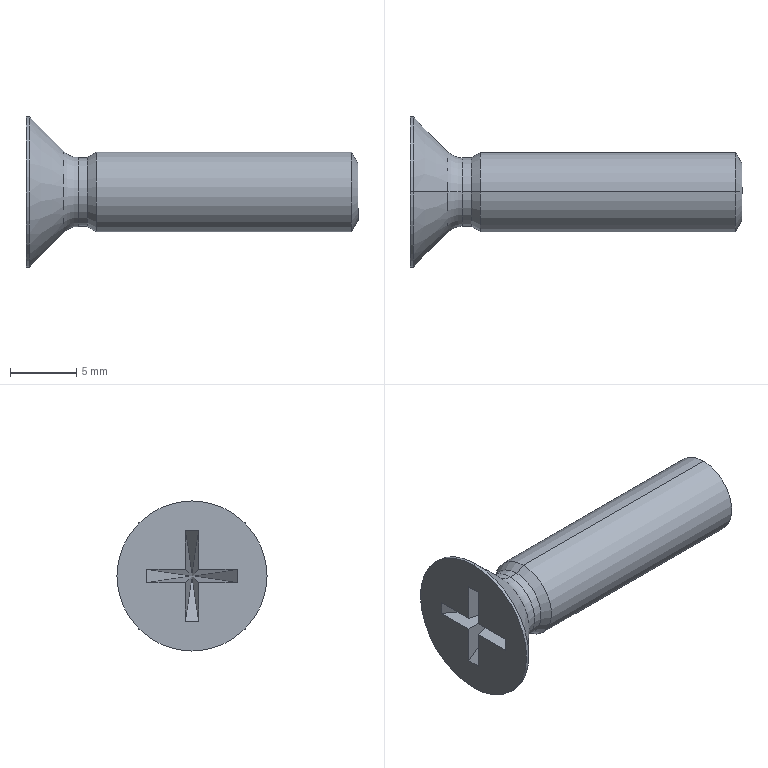Part | SolidWorks | features BaseBody 1 | 1 solid | 28 faces | box 25 x 11.3 x 11.3 mm | volume 779.668 mm3 | plane 14 | cone 6 | cylinder 6 | torus 2 | commonest cylinder face diameters 5.196 x2 6 x2 11.3 x2
STEP:
#1=CARTESIAN_POINT('',(0.,3.4,0.5));
#2=VERTEX_POINT('',#1);
#3=CARTESIAN_POINT('',(3.5,0.,0.));
#4=VERTEX_POINT('',#3);
#5=CARTESIAN_POINT('',(0.,3.4,0.5));
#6=DIRECTION('',(0.7135,-0.6932,-0.1019));
#7=VECTOR('',#6,1000.);
#8=LINE('',#5,#7);
#9=EDGE_CURVE('',#2,#4,#8,.T.);
#10=ORIENTED_EDGE('',*,*,#9,.F.);
#11=CARTESIAN_POINT('',(0.,3.4,-0.5));
#12=VERTEX_POINT('',#11);
#13=CARTESIAN_POINT('',(0.,3.4,0.5));
#14=DIRECTION('',(0.,0.,-1.));
#15=VECTOR('',#14,1000.);
#16=LINE('',#13,#15);
#17=EDGE_CURVE('',#2,#12,#16,.T.);
#18=ORIENTED_EDGE('',*,*,#17,.T.);
#19=CARTESIAN_POINT('',(0.,3.4,-0.5));
#20=DIRECTION('',(0.7135,-0.6932,0.1019));
#21=VECTOR('',#20,1000.);
#22=LINE('',#19,#21);
#23=EDGE_CURVE('',#12,#4,#22,.T.);
#24=ORIENTED_EDGE('',*,*,#23,.T.);
#25=EDGE_LOOP('',(#10,#18,#24));
#26=FACE_OUTER_BOUND('',#25,.T.);
#27=CARTESIAN_POINT('',(0.,3.4,0.5));
#28=DIRECTION('',(0.6968,0.7173,0.));
#29=DIRECTION('',(0.,0.,-1.));
#30=AXIS2_PLACEMENT_3D('',#27,#28,#29);
#31=PLANE('',#30);
#32=ADVANCED_FACE('',(#26),#31,.F.);
#33=ORIENTED_EDGE('',*,*,#23,.F.);
#34=CARTESIAN_POINT('',(0.,0.5,-0.5));
#35=VERTEX_POINT('',#34);
#36=CARTESIAN_POINT('',(0.,3.4,-0.5));
#37=DIRECTION('',(0.,-1.,0.));
#38=VECTOR('',#37,1000.);
#39=LINE('',#36,#38);
#40=EDGE_CURVE('',#12,#35,#39,.T.);
#41=ORIENTED_EDGE('',*,*,#40,.T.);
#42=CARTESIAN_POINT('',(3.5,0.,0.));
#43=DIRECTION('',(-0.9802,0.14,-0.14));
#44=VECTOR('',#43,1000.);
#45=LINE('',#42,#44);
#46=EDGE_CURVE('',#4,#35,#45,.T.);
#47=ORIENTED_EDGE('',*,*,#46,.F.);
#48=EDGE_LOOP('',(#33,#41,#47));
#49=FACE_OUTER_BOUND('',#48,.T.);
#50=CARTESIAN_POINT('',(3.5,0.,0.));
#51=DIRECTION('',(-0.1414,0.,0.9899));
#52=DIRECTION('',(0.,1.,0.));
#53=AXIS2_PLACEMENT_3D('',#50,#51,#52);
#54=PLANE('',#53);
#55=ADVANCED_FACE('',(#49),#54,.T.);
#56=CARTESIAN_POINT('',(0.,0.5,0.5));
#57=VERTEX_POINT('',#56);
#58=CARTESIAN_POINT('',(0.,3.4,0.5));
#59=DIRECTION('',(0.,1.,0.));
#60=VECTOR('',#59,1000.);
#61=LINE('',#58,#60);
#62=EDGE_CURVE('',#57,#2,#61,.T.);
#63=ORIENTED_EDGE('',*,*,#62,.T.);
#64=ORIENTED_EDGE('',*,*,#9,.T.);
#65=CARTESIAN_POINT('',(3.5,0.,0.));
#66=DIRECTION('',(0.9802,-0.14,-0.14));
#67=VECTOR('',#66,1000.);
#68=LINE('',#65,#67);
#69=EDGE_CURVE('',#57,#4,#68,.T.);
#70=ORIENTED_EDGE('',*,*,#69,.F.);
#71=EDGE_LOOP('',(#63,#64,#70));
#72=FACE_OUTER_BOUND('',#71,.T.);
#73=CARTESIAN_POINT('',(3.5,0.,0.));
#74=DIRECTION('',(-0.1414,0.,-0.9899));
#75=DIRECTION('',(-0.9899,0.,0.1414));
#76=AXIS2_PLACEMENT_3D('',#73,#74,#75);
#77=PLANE('',#76);
#78=ADVANCED_FACE('',(#72),#77,.T.);
#79=CARTESIAN_POINT('',(0.,-3.4,-0.5));
#80=VERTEX_POINT('',#79);
#81=CARTESIAN_POINT('',(0.,-3.4,-0.5));
#82=DIRECTION('',(0.7135,0.6932,0.1019));
#83=VECTOR('',#82,1000.);
#84=LINE('',#81,#83);
#85=EDGE_CURVE('',#80,#4,#84,.T.);
#86=ORIENTED_EDGE('',*,*,#85,.F.);
#87=CARTESIAN_POINT('',(0.,-3.4,0.5));
#88=VERTEX_POINT('',#87);
#89=CARTESIAN_POINT('',(0.,-3.4,0.5));
#90=DIRECTION('',(0.,0.,1.));
#91=VECTOR('',#90,1000.);
#92=LINE('',#89,#91);
#93=EDGE_CURVE('',#80,#88,#92,.T.);
#94=ORIENTED_EDGE('',*,*,#93,.T.);
#95=CARTESIAN_POINT('',(0.,-3.4,0.5));
#96=DIRECTION('',(0.7135,0.6932,-0.1019));
#97=VECTOR('',#96,1000.);
#98=LINE('',#95,#97);
#99=EDGE_CURVE('',#88,#4,#98,.T.);
#100=ORIENTED_EDGE('',*,*,#99,.T.);
#101=EDGE_LOOP('',(#86,#94,#100));
#102=FACE_OUTER_BOUND('',#101,.T.);
#103=CARTESIAN_POINT('',(0.,-3.4,-0.5));
#104=DIRECTION('',(0.6968,-0.7173,0.));
#105=DIRECTION('',(0.,0.,-1.));
#106=AXIS2_PLACEMENT_3D('',#103,#104,#105);
#107=PLANE('',#106);
#108=ADVANCED_FACE('',(#102),#107,.F.);
#109=CARTESIAN_POINT('',(0.,-0.5,-0.5));
#110=VERTEX_POINT('',#109);
#111=CARTESIAN_POINT('',(0.,3.4,-0.5));
#112=DIRECTION('',(0.,-1.,0.));
#113=VECTOR('',#112,1000.);
#114=LINE('',#111,#113);
#115=EDGE_CURVE('',#110,#80,#114,.T.);
#116=ORIENTED_EDGE('',*,*,#115,.T.);
#117=ORIENTED_EDGE('',*,*,#85,.T.);
#118=CARTESIAN_POINT('',(3.5,0.,0.));
#119=DIRECTION('',(0.9802,0.14,0.14));
#120=VECTOR('',#119,1000.);
#121=LINE('',#118,#120);
#122=EDGE_CURVE('',#110,#4,#121,.T.);
#123=ORIENTED_EDGE('',*,*,#122,.F.);
#124=EDGE_LOOP('',(#116,#117,#123));
#125=FACE_OUTER_BOUND('',#124,.T.);
#126=CARTESIAN_POINT('',(3.5,0.,0.));
#127=DIRECTION('',(-0.1414,0.,0.9899));
#128=DIRECTION('',(0.,1.,0.));
#129=AXIS2_PLACEMENT_3D('',#126,#127,#128);
#130=PLANE('',#129);
#131=ADVANCED_FACE('',(#125),#130,.T.);
#132=ORIENTED_EDGE('',*,*,#99,.F.);
#133=CARTESIAN_POINT('',(0.,-0.5,0.5));
#134=VERTEX_POINT('',#133);
#135=CARTESIAN_POINT('',(0.,3.4,0.5));
#136=DIRECTION('',(0.,1.,0.));
#137=VECTOR('',#136,1000.);
#138=LINE('',#135,#137);
#139=EDGE_CURVE('',#88,#134,#138,.T.);
#140=ORIENTED_EDGE('',*,*,#139,.T.);
#141=CARTESIAN_POINT('',(3.5,0.,0.));
#142=DIRECTION('',(-0.9802,-0.14,0.14));
#143=VECTOR('',#142,1000.);
#144=LINE('',#141,#143);
#145=EDGE_CURVE('',#4,#134,#144,.T.);
#146=ORIENTED_EDGE('',*,*,#145,.F.);
#147=EDGE_LOOP('',(#132,#140,#146));
#148=FACE_OUTER_BOUND('',#147,.T.);
#149=CARTESIAN_POINT('',(3.5,0.,0.));
#150=DIRECTION('',(-0.1414,0.,-0.9899));
#151=DIRECTION('',(-0.9899,0.,0.1414));
#152=AXIS2_PLACEMENT_3D('',#149,#150,#151);
#153=PLANE('',#152);
#154=ADVANCED_FACE('',(#148),#153,.T.);
#155=CARTESIAN_POINT('',(0.,-0.5,3.4));
#156=VERTEX_POINT('',#155);
#157=CARTESIAN_POINT('',(0.,-0.5,3.4));
#158=DIRECTION('',(0.7135,0.1019,-0.6932));
#159=VECTOR('',#158,1000.);
#160=LINE('',#157,#159);
#161=EDGE_CURVE('',#156,#4,#160,.T.);
#162=ORIENTED_EDGE('',*,*,#161,.F.);
#163=CARTESIAN_POINT('',(0.,0.5,3.4));
#164=VERTEX_POINT('',#163);
#165=CARTESIAN_POINT('',(0.,0.5,3.4));
#166=DIRECTION('',(0.,1.,0.));
#167=VECTOR('',#166,1000.);
#168=LINE('',#165,#167);
#169=EDGE_CURVE('',#156,#164,#168,.T.);
#170=ORIENTED_EDGE('',*,*,#169,.T.);
#171=CARTESIAN_POINT('',(0.,0.5,3.4));
#172=DIRECTION('',(0.7135,-0.1019,-0.6932));
#173=VECTOR('',#172,1000.);
#174=LINE('',#171,#173);
#175=EDGE_CURVE('',#164,#4,#174,.T.);
#176=ORIENTED_EDGE('',*,*,#175,.T.);
#177=EDGE_LOOP('',(#162,#170,#176));
#178=FACE_OUTER_BOUND('',#177,.T.);
#179=CARTESIAN_POINT('',(0.,-0.5,3.4));
#180=DIRECTION('',(0.6968,0.,0.7173));
#181=DIRECTION('',(0.,-1.,0.));
#182=AXIS2_PLACEMENT_3D('',#179,#180,#181);
#183=PLANE('',#182);
#184=ADVANCED_FACE('',(#178),#183,.F.);
#185=CARTESIAN_POINT('',(0.,0.5,-3.4));
#186=VERTEX_POINT('',#185);
#187=CARTESIAN_POINT('',(0.,0.5,-3.4));
#188=DIRECTION('',(0.7135,-0.1019,0.6932));
#189=VECTOR('',#188,1000.);
#190=LINE('',#187,#189);
#191=EDGE_CURVE('',#186,#4,#190,.T.);
#192=ORIENTED_EDGE('',*,*,#191,.F.);
#193=CARTESIAN_POINT('',(0.,-0.5,-3.4));
#194=VERTEX_POINT('',#193);
#195=CARTESIAN_POINT('',(0.,0.5,-3.4));
#196=DIRECTION('',(0.,-1.,0.));
#197=VECTOR('',#196,1000.);
#198=LINE('',#195,#197);
#199=EDGE_CURVE('',#186,#194,#198,.T.);
#200=ORIENTED_EDGE('',*,*,#199,.T.);
#201=CARTESIAN_POINT('',(0.,-0.5,-3.4));
#202=DIRECTION('',(0.7135,0.1019,0.6932));
#203=VECTOR('',#202,1000.);
#204=LINE('',#201,#203);
#205=EDGE_CURVE('',#194,#4,#204,.T.);
#206=ORIENTED_EDGE('',*,*,#205,.T.);
#207=EDGE_LOOP('',(#192,#200,#206));
#208=FACE_OUTER_BOUND('',#207,.T.);
#209=CARTESIAN_POINT('',(0.,0.5,-3.4));
#210=DIRECTION('',(0.6968,0.,-0.7173));
#211=DIRECTION('',(0.,-1.,0.));
#212=AXIS2_PLACEMENT_3D('',#209,#210,#211);
#213=PLANE('',#212);
#214=ADVANCED_FACE('',(#208),#213,.F.);
#215=CARTESIAN_POINT('',(25.,0.,2.134));
#216=VERTEX_POINT('',#215);
#217=CARTESIAN_POINT('',(25.,0.,-2.134));
#218=VERTEX_POINT('',#217);
#219=CARTESIAN_POINT('',(25.,0.,0.));
#220=DIRECTION('',(1.,0.,0.));
#221=DIRECTION('',(0.,0.,-1.));
#222=AXIS2_PLACEMENT_3D('',#219,#220,#221);
#223=CIRCLE('',#222,2.134);
#224=EDGE_CURVE('',#216,#218,#223,.T.);
#225=ORIENTED_EDGE('',*,*,#224,.T.);
#226=CARTESIAN_POINT('',(25.,0.,0.));
#227=DIRECTION('',(1.,0.,0.));
#228=DIRECTION('',(0.,0.,-1.));
#229=AXIS2_PLACEMENT_3D('',#226,#227,#228);
#230=CIRCLE('',#229,2.134);
#231=EDGE_CURVE('',#218,#216,#230,.T.);
#232=ORIENTED_EDGE('',*,*,#231,.T.);
#233=EDGE_LOOP('',(#225,#232));
#234=FACE_OUTER_BOUND('',#233,.T.);
#235=CARTESIAN_POINT('',(25.,3.,0.));
#236=DIRECTION('',(-1.,0.,0.));
#237=DIRECTION('',(0.,0.,1.));
#238=AXIS2_PLACEMENT_3D('',#235,#236,#237);
#239=PLANE('',#238);
#240=ADVANCED_FACE('',(#234),#239,.F.);
#241=CARTESIAN_POINT('',(24.505,0.,-3.));
#242=VERTEX_POINT('',#241);
#243=CARTESIAN_POINT('',(24.505,0.,-3.));
#244=DIRECTION('',(-0.4959,0.,-0.8684));
#245=VECTOR('',#244,1000.);
#246=LINE('',#243,#245);
#247=EDGE_CURVE('',#218,#242,#246,.T.);
#248=ORIENTED_EDGE('',*,*,#247,.F.);
#249=ORIENTED_EDGE('',*,*,#224,.F.);
#250=CARTESIAN_POINT('',(24.505,0.,3.));
#251=VERTEX_POINT('',#250);
#252=CARTESIAN_POINT('',(24.505,0.,3.));
#253=DIRECTION('',(-0.4959,0.,0.8684));
#254=VECTOR('',#253,1000.);
#255=LINE('',#252,#254);
#256=EDGE_CURVE('',#216,#251,#255,.T.);
#257=ORIENTED_EDGE('',*,*,#256,.T.);
#258=CARTESIAN_POINT('',(24.505,0.,0.));
#259=DIRECTION('',(1.,0.,0.));
#260=DIRECTION('',(0.,0.,-1.));
#261=AXIS2_PLACEMENT_3D('',#258,#259,#260);
#262=CIRCLE('',#261,3.);
#263=EDGE_CURVE('',#251,#242,#262,.T.);
#264=ORIENTED_EDGE('',*,*,#263,.T.);
#265=EDGE_LOOP('',(#248,#249,#257,#264));
#266=FACE_OUTER_BOUND('',#265,.T.);
#267=CARTESIAN_POINT('',(24.505,0.,0.));
#268=DIRECTION('',(-1.,0.,0.));
#269=DIRECTION('',(0.,0.,1.));
#270=AXIS2_PLACEMENT_3D('',#267,#268,#269);
#271=CONICAL_SURFACE('',#270,3.,1.052);
#272=ADVANCED_FACE('',(#266),#271,.T.);
#273=CARTESIAN_POINT('',(5.3,0.,-3.));
#274=VERTEX_POINT('',#273);
#275=CARTESIAN_POINT('',(0.,0.,-3.));
#276=DIRECTION('',(-1.,0.,0.));
#277=VECTOR('',#276,1000.);
#278=LINE('',#275,#277);
#279=EDGE_CURVE('',#242,#274,#278,.T.);
#280=ORIENTED_EDGE('',*,*,#279,.F.);
#281=ORIENTED_EDGE('',*,*,#263,.F.);
#282=CARTESIAN_POINT('',(5.3,0.,3.));
#283=VERTEX_POINT('',#282);
#284=CARTESIAN_POINT('',(0.,0.,3.));
#285=DIRECTION('',(-1.,0.,0.));
#286=VECTOR('',#285,1000.);
#287=LINE('',#284,#286);
#288=EDGE_CURVE('',#251,#283,#287,.T.);
#289=ORIENTED_EDGE('',*,*,#288,.T.);
#290=CARTESIAN_POINT('',(5.3,0.,0.));
#291=DIRECTION('',(-1.,0.,0.));
#292=DIRECTION('',(0.,0.,1.));
#293=AXIS2_PLACEMENT_3D('',#290,#291,#292);
#294=CIRCLE('',#293,3.);
#295=EDGE_CURVE('',#274,#283,#294,.T.);
#296=ORIENTED_EDGE('',*,*,#295,.F.);
#297=EDGE_LOOP('',(#280,#281,#289,#296));
#298=FACE_OUTER_BOUND('',#297,.T.);
#299=CARTESIAN_POINT('',(0.,0.,0.));
#300=DIRECTION('',(-1.,0.,0.));
#301=DIRECTION('',(0.,0.,1.));
#302=AXIS2_PLACEMENT_3D('',#299,#300,#301);
#303=CYLINDRICAL_SURFACE('',#302,3.);
#304=ADVANCED_FACE('',(#298),#303,.T.);
#305=CARTESIAN_POINT('',(4.604,0.,2.598));
#306=VERTEX_POINT('',#305);
#307=CARTESIAN_POINT('',(5.3,0.,3.));
#308=DIRECTION('',(0.866,0.,0.5));
#309=VECTOR('',#308,1000.);
#310=LINE('',#307,#309);
#311=EDGE_CURVE('',#306,#283,#310,.T.);
#312=ORIENTED_EDGE('',*,*,#311,.F.);
#313=CARTESIAN_POINT('',(4.604,0.,-2.598));
#314=VERTEX_POINT('',#313);
#315=CARTESIAN_POINT('',(4.604,0.,0.));
#316=DIRECTION('',(-1.,0.,0.));
#317=DIRECTION('',(0.,0.,1.));
#318=AXIS2_PLACEMENT_3D('',#315,#316,#317);
#319=CIRCLE('',#318,2.598);
#320=EDGE_CURVE('',#314,#306,#319,.T.);
#321=ORIENTED_EDGE('',*,*,#320,.F.);
#322=CARTESIAN_POINT('',(5.3,0.,-3.));
#323=DIRECTION('',(0.866,0.,-0.5));
#324=VECTOR('',#323,1000.);
#325=LINE('',#322,#324);
#326=EDGE_CURVE('',#314,#274,#325,.T.);
#327=ORIENTED_EDGE('',*,*,#326,.T.);
#328=ORIENTED_EDGE('',*,*,#295,.T.);
#329=EDGE_LOOP('',(#312,#321,#327,#328));
#330=FACE_OUTER_BOUND('',#329,.T.);
#331=CARTESIAN_POINT('',(5.3,0.,0.));
#332=DIRECTION('',(1.,0.,0.));
#333=DIRECTION('',(0.,0.,-1.));
#334=AXIS2_PLACEMENT_3D('',#331,#332,#333);
#335=CONICAL_SURFACE('',#334,3.,0.5236);
#336=ADVANCED_FACE('',(#330),#335,.T.);
#337=CARTESIAN_POINT('',(3.921,0.,-2.598));
#338=VERTEX_POINT('',#337);
#339=CARTESIAN_POINT('',(0.,0.,-2.598));
#340=DIRECTION('',(-1.,0.,0.));
#341=VECTOR('',#340,1000.);
#342=LINE('',#339,#341);
#343=EDGE_CURVE('',#314,#338,#342,.T.);
#344=ORIENTED_EDGE('',*,*,#343,.F.);
#345=ORIENTED_EDGE('',*,*,#320,.T.);
#346=CARTESIAN_POINT('',(3.921,0.,2.598));
#347=VERTEX_POINT('',#346);
#348=CARTESIAN_POINT('',(0.,0.,2.598));
#349=DIRECTION('',(-1.,0.,0.));
#350=VECTOR('',#349,1000.);
#351=LINE('',#348,#350);
#352=EDGE_CURVE('',#306,#347,#351,.T.);
#353=ORIENTED_EDGE('',*,*,#352,.T.);
#354=CARTESIAN_POINT('',(3.921,0.,0.));
#355=DIRECTION('',(-1.,0.,0.));
#356=DIRECTION('',(0.,0.,1.));
#357=AXIS2_PLACEMENT_3D('',#354,#355,#356);
#358=CIRCLE('',#357,2.598);
#359=EDGE_CURVE('',#338,#347,#358,.T.);
#360=ORIENTED_EDGE('',*,*,#359,.F.);
#361=EDGE_LOOP('',(#344,#345,#353,#360));
#362=FACE_OUTER_BOUND('',#361,.T.);
#363=CARTESIAN_POINT('',(0.,0.,0.));
#364=DIRECTION('',(-1.,0.,0.));
#365=DIRECTION('',(0.,0.,1.));
#366=AXIS2_PLACEMENT_3D('',#363,#364,#365);
#367=CYLINDRICAL_SURFACE('',#366,2.598);
#368=ADVANCED_FACE('',(#362),#367,.T.);
#369=CARTESIAN_POINT('',(2.861,0.,-3.037));
#370=VERTEX_POINT('',#369);
#371=CARTESIAN_POINT('',(3.921,0.,-4.098));
#372=DIRECTION('',(0.,1.,0.));
#373=DIRECTION('',(0.,0.,1.));
#374=AXIS2_PLACEMENT_3D('',#371,#372,#373);
#375=CIRCLE('',#374,1.5);
#376=EDGE_CURVE('',#370,#338,#375,.T.);
#377=ORIENTED_EDGE('',*,*,#376,.F.);
#378=CARTESIAN_POINT('',(2.861,0.,3.037));
#379=VERTEX_POINT('',#378);
#380=CARTESIAN_POINT('',(2.861,0.,0.));
#381=DIRECTION('',(-1.,0.,0.));
#382=DIRECTION('',(0.,0.,1.));
#383=AXIS2_PLACEMENT_3D('',#380,#381,#382);
#384=CIRCLE('',#383,3.037);
#385=EDGE_CURVE('',#379,#370,#384,.T.);
#386=ORIENTED_EDGE('',*,*,#385,.F.);
#387=CARTESIAN_POINT('',(3.921,0.,4.098));
#388=DIRECTION('',(0.,-1.,0.));
#389=DIRECTION('',(0.,0.,-1.));
#390=AXIS2_PLACEMENT_3D('',#387,#388,#389);
#391=CIRCLE('',#390,1.5);
#392=EDGE_CURVE('',#379,#347,#391,.T.);
#393=ORIENTED_EDGE('',*,*,#392,.T.);
#394=CARTESIAN_POINT('',(3.921,0.,0.));
#395=DIRECTION('',(-1.,0.,0.));
#396=DIRECTION('',(0.,0.,1.));
#397=AXIS2_PLACEMENT_3D('',#394,#395,#396);
#398=CIRCLE('',#397,2.598);
#399=EDGE_CURVE('',#347,#338,#398,.T.);
#400=ORIENTED_EDGE('',*,*,#399,.T.);
#401=EDGE_LOOP('',(#377,#386,#393,#400));
#402=FACE_OUTER_BOUND('',#401,.T.);
#403=CARTESIAN_POINT('',(3.921,0.,0.));
#404=DIRECTION('',(-1.,0.,0.));
#405=DIRECTION('',(0.,0.,1.));
#406=AXIS2_PLACEMENT_3D('',#403,#404,#405);
#407=TOROIDAL_SURFACE('',#406,4.098,1.5);
#408=ADVANCED_FACE('',(#402),#407,.F.);
#409=CARTESIAN_POINT('',(0.248,0.,-5.65));
#410=VERTEX_POINT('',#409);
#411=CARTESIAN_POINT('',(2.861,0.,-3.037));
#412=DIRECTION('',(-0.7071,0.,-0.7071));
#413=VECTOR('',#412,1000.);
#414=LINE('',#411,#413);
#415=EDGE_CURVE('',#370,#410,#414,.T.);
#416=ORIENTED_EDGE('',*,*,#415,.F.);
#417=CARTESIAN_POINT('',(2.861,0.,0.));
#418=DIRECTION('',(-1.,0.,0.));
#419=DIRECTION('',(0.,0.,1.));
#420=AXIS2_PLACEMENT_3D('',#417,#418,#419);
#421=CIRCLE('',#420,3.037);
#422=EDGE_CURVE('',#370,#379,#421,.T.);
#423=ORIENTED_EDGE('',*,*,#422,.T.);
#424=CARTESIAN_POINT('',(0.248,0.,5.65));
#425=VERTEX_POINT('',#424);
#426=CARTESIAN_POINT('',(2.861,0.,3.037));
#427=DIRECTION('',(-0.7071,0.,0.7071));
#428=VECTOR('',#427,1000.);
#429=LINE('',#426,#428);
#430=EDGE_CURVE('',#379,#425,#429,.T.);
#431=ORIENTED_EDGE('',*,*,#430,.T.);
#432=CARTESIAN_POINT('',(0.248,0.,0.));
#433=DIRECTION('',(-1.,0.,0.));
#434=DIRECTION('',(0.,0.,1.));
#435=AXIS2_PLACEMENT_3D('',#432,#433,#434);
#436=CIRCLE('',#435,5.65);
#437=EDGE_CURVE('',#410,#425,#436,.T.);
#438=ORIENTED_EDGE('',*,*,#437,.F.);
#439=EDGE_LOOP('',(#416,#423,#431,#438));
#440=FACE_OUTER_BOUND('',#439,.T.);
#441=CARTESIAN_POINT('',(2.861,0.,0.));
#442=DIRECTION('',(-1.,0.,0.));
#443=DIRECTION('',(0.,0.,1.));
#444=AXIS2_PLACEMENT_3D('',#441,#442,#443);
#445=CONICAL_SURFACE('',#444,3.037,0.7854);
#446=ADVANCED_FACE('',(#440),#445,.T.);
#447=CARTESIAN_POINT('',(0.,0.,-5.65));
#448=VERTEX_POINT('',#447);
#449=CARTESIAN_POINT('',(0.,0.,-5.65));
#450=DIRECTION('',(-1.,0.,0.));
#451=VECTOR('',#450,1000.);
#452=LINE('',#449,#451);
#453=EDGE_CURVE('',#410,#448,#452,.T.);
#454=ORIENTED_EDGE('',*,*,#453,.F.);
#455=ORIENTED_EDGE('',*,*,#437,.T.);
#456=CARTESIAN_POINT('',(0.,0.,5.65));
#457=VERTEX_POINT('',#456);
#458=CARTESIAN_POINT('',(0.,0.,5.65));
#459=DIRECTION('',(-1.,0.,0.));
#460=VECTOR('',#459,1000.);
#461=LINE('',#458,#460);
#462=EDGE_CURVE('',#425,#457,#461,.T.);
#463=ORIENTED_EDGE('',*,*,#462,.T.);
#464=CARTESIAN_POINT('',(0.,0.,0.));
#465=DIRECTION('',(-1.,0.,0.));
#466=DIRECTION('',(0.,0.,1.));
#467=AXIS2_PLACEMENT_3D('',#464,#465,#466);
#468=CIRCLE('',#467,5.65);
#469=EDGE_CURVE('',#448,#457,#468,.T.);
#470=ORIENTED_EDGE('',*,*,#469,.F.);
#471=EDGE_LOOP('',(#454,#455,#463,#470));
#472=FACE_OUTER_BOUND('',#471,.T.);
#473=CARTESIAN_POINT('',(0.,0.,0.));
#474=DIRECTION('',(-1.,0.,0.));
#475=DIRECTION('',(0.,0.,1.));
#476=AXIS2_PLACEMENT_3D('',#473,#474,#475);
#477=CYLINDRICAL_SURFACE('',#476,5.65);
#478=ADVANCED_FACE('',(#472),#477,.T.);
#479=CARTESIAN_POINT('',(0.,-0.5,-3.4));
#480=DIRECTION('',(0.,0.,1.));
#481=VECTOR('',#480,1000.);
#482=LINE('',#479,#481);
#483=EDGE_CURVE('',#194,#110,#482,.T.);
#484=ORIENTED_EDGE('',*,*,#483,.T.);
#485=ORIENTED_EDGE('',*,*,#122,.T.);
#486=ORIENTED_EDGE('',*,*,#205,.F.);
#487=EDGE_LOOP('',(#484,#485,#486));
#488=FACE_OUTER_BOUND('',#487,.T.);
#489=CARTESIAN_POINT('',(3.5,0.,0.));
#490=DIRECTION('',(-0.1414,0.9899,0.));
#491=DIRECTION('',(0.,0.,1.));
#492=AXIS2_PLACEMENT_3D('',#489,#490,#491);
#493=PLANE('',#492);
#494=ADVANCED_FACE('',(#488),#493,.T.);
#495=ORIENTED_EDGE('',*,*,#161,.T.);
#496=ORIENTED_EDGE('',*,*,#145,.T.);
#497=CARTESIAN_POINT('',(0.,-0.5,-3.4));
#498=DIRECTION('',(0.,0.,1.));
#499=VECTOR('',#498,1000.);
#500=LINE('',#497,#499);
#501=EDGE_CURVE('',#134,#156,#500,.T.);
#502=ORIENTED_EDGE('',*,*,#501,.T.);
#503=EDGE_LOOP('',(#495,#496,#502));
#504=FACE_OUTER_BOUND('',#503,.T.);
#505=CARTESIAN_POINT('',(3.5,0.,0.));
#506=DIRECTION('',(-0.1414,0.9899,0.));
#507=DIRECTION('',(0.,0.,1.));
#508=AXIS2_PLACEMENT_3D('',#505,#506,#507);
#509=PLANE('',#508);
#510=ADVANCED_FACE('',(#504),#509,.T.);
#511=ORIENTED_EDGE('',*,*,#191,.T.);
#512=ORIENTED_EDGE('',*,*,#46,.T.);
#513=CARTESIAN_POINT('',(0.,0.5,-3.4));
#514=DIRECTION('',(0.,0.,-1.));
#515=VECTOR('',#514,1000.);
#516=LINE('',#513,#515);
#517=EDGE_CURVE('',#35,#186,#516,.T.);
#518=ORIENTED_EDGE('',*,*,#517,.T.);
#519=EDGE_LOOP('',(#511,#512,#518));
#520=FACE_OUTER_BOUND('',#519,.T.);
#521=CARTESIAN_POINT('',(3.5,0.,0.));
#522=DIRECTION('',(-0.1414,-0.9899,0.));
#523=DIRECTION('',(-0.9899,0.1414,0.));
#524=AXIS2_PLACEMENT_3D('',#521,#522,#523);
#525=PLANE('',#524);
#526=ADVANCED_FACE('',(#520),#525,.T.);
#527=CARTESIAN_POINT('',(0.,0.5,-3.4));
#528=DIRECTION('',(0.,0.,-1.));
#529=VECTOR('',#528,1000.);
#530=LINE('',#527,#529);
#531=EDGE_CURVE('',#164,#57,#530,.T.);
#532=ORIENTED_EDGE('',*,*,#531,.T.);
#533=ORIENTED_EDGE('',*,*,#69,.T.);
#534=ORIENTED_EDGE('',*,*,#175,.F.);
#535=EDGE_LOOP('',(#532,#533,#534));
#536=FACE_OUTER_BOUND('',#535,.T.);
#537=CARTESIAN_POINT('',(3.5,0.,0.));
#538=DIRECTION('',(-0.1414,-0.9899,0.));
#539=DIRECTION('',(-0.9899,0.1414,0.));
#540=AXIS2_PLACEMENT_3D('',#537,#538,#539);
#541=PLANE('',#540);
#542=ADVANCED_FACE('',(#536),#541,.T.);
#543=ORIENTED_EDGE('',*,*,#62,.F.);
#544=ORIENTED_EDGE('',*,*,#531,.F.);
#545=ORIENTED_EDGE('',*,*,#169,.F.);
#546=ORIENTED_EDGE('',*,*,#501,.F.);
#547=ORIENTED_EDGE('',*,*,#139,.F.);
#548=ORIENTED_EDGE('',*,*,#93,.F.);
#549=ORIENTED_EDGE('',*,*,#115,.F.);
#550=ORIENTED_EDGE('',*,*,#483,.F.);
#551=ORIENTED_EDGE('',*,*,#199,.F.);
#552=ORIENTED_EDGE('',*,*,#517,.F.);
#553=ORIENTED_EDGE('',*,*,#40,.F.);
#554=ORIENTED_EDGE('',*,*,#17,.F.);
#555=EDGE_LOOP('',(#543,#544,#545,#546,#547,#548,#549,#550,#551,#552,#553,#554));
#556=FACE_BOUND('',#555,.T.);
#557=CARTESIAN_POINT('',(0.,0.,0.));
#558=DIRECTION('',(-1.,0.,0.));
#559=DIRECTION('',(0.,0.,1.));
#560=AXIS2_PLACEMENT_3D('',#557,#558,#559);
#561=CIRCLE('',#560,5.65);
#562=EDGE_CURVE('',#457,#448,#561,.T.);
#563=ORIENTED_EDGE('',*,*,#562,.T.);
#564=ORIENTED_EDGE('',*,*,#469,.T.);
#565=EDGE_LOOP('',(#563,#564));
#566=FACE_OUTER_BOUND('',#565,.T.);
#567=CARTESIAN_POINT('',(0.,0.,0.));
#568=DIRECTION('',(1.,0.,0.));
#569=DIRECTION('',(0.,0.,1.));
#570=AXIS2_PLACEMENT_3D('',#567,#568,#569);
#571=PLANE('',#570);
#572=ADVANCED_FACE('',(#556,#566),#571,.F.);
#573=CARTESIAN_POINT('',(0.248,0.,0.));
#574=DIRECTION('',(-1.,0.,0.));
#575=DIRECTION('',(0.,0.,1.));
#576=AXIS2_PLACEMENT_3D('',#573,#574,#575);
#577=CIRCLE('',#576,5.65);
#578=EDGE_CURVE('',#425,#410,#577,.T.);
#579=ORIENTED_EDGE('',*,*,#578,.T.);
#580=ORIENTED_EDGE('',*,*,#453,.T.);
#581=ORIENTED_EDGE('',*,*,#562,.F.);
#582=ORIENTED_EDGE('',*,*,#462,.F.);
#583=EDGE_LOOP('',(#579,#580,#581,#582));
#584=FACE_OUTER_BOUND('',#583,.T.);
#585=CARTESIAN_POINT('',(0.,0.,0.));
#586=DIRECTION('',(-1.,0.,0.));
#587=DIRECTION('',(0.,0.,1.));
#588=AXIS2_PLACEMENT_3D('',#585,#586,#587);
#589=CYLINDRICAL_SURFACE('',#588,5.65);
#590=ADVANCED_FACE('',(#584),#589,.T.);
#591=ORIENTED_EDGE('',*,*,#385,.T.);
#592=ORIENTED_EDGE('',*,*,#415,.T.);
#593=ORIENTED_EDGE('',*,*,#578,.F.);
#594=ORIENTED_EDGE('',*,*,#430,.F.);
#595=EDGE_LOOP('',(#591,#592,#593,#594));
#596=FACE_OUTER_BOUND('',#595,.T.);
#597=CARTESIAN_POINT('',(2.861,0.,0.));
#598=DIRECTION('',(-1.,0.,0.));
#599=DIRECTION('',(0.,0.,1.));
#600=AXIS2_PLACEMENT_3D('',#597,#598,#599);
#601=CONICAL_SURFACE('',#600,3.037,0.7854);
#602=ADVANCED_FACE('',(#596),#601,.T.);
#603=ORIENTED_EDGE('',*,*,#422,.F.);
#604=ORIENTED_EDGE('',*,*,#376,.T.);
#605=ORIENTED_EDGE('',*,*,#359,.T.);
#606=ORIENTED_EDGE('',*,*,#392,.F.);
#607=EDGE_LOOP('',(#603,#604,#605,#606));
#608=FACE_OUTER_BOUND('',#607,.T.);
#609=CARTESIAN_POINT('',(3.921,0.,0.));
#610=DIRECTION('',(-1.,0.,0.));
#611=DIRECTION('',(0.,0.,1.));
#612=AXIS2_PLACEMENT_3D('',#609,#610,#611);
#613=TOROIDAL_SURFACE('',#612,4.098,1.5);
#614=ADVANCED_FACE('',(#608),#613,.F.);
#615=CARTESIAN_POINT('',(4.604,0.,0.));
#616=DIRECTION('',(-1.,0.,0.));
#617=DIRECTION('',(0.,0.,1.));
#618=AXIS2_PLACEMENT_3D('',#615,#616,#617);
#619=CIRCLE('',#618,2.598);
#620=EDGE_CURVE('',#306,#314,#619,.T.);
#621=ORIENTED_EDGE('',*,*,#620,.T.);
#622=ORIENTED_EDGE('',*,*,#343,.T.);
#623=ORIENTED_EDGE('',*,*,#399,.F.);
#624=ORIENTED_EDGE('',*,*,#352,.F.);
#625=EDGE_LOOP('',(#621,#622,#623,#624));
#626=FACE_OUTER_BOUND('',#625,.T.);
#627=CARTESIAN_POINT('',(0.,0.,0.));
#628=DIRECTION('',(-1.,0.,0.));
#629=DIRECTION('',(0.,0.,1.));
#630=AXIS2_PLACEMENT_3D('',#627,#628,#629);
#631=CYLINDRICAL_SURFACE('',#630,2.598);
#632=ADVANCED_FACE('',(#626),#631,.T.);
#633=ORIENTED_EDGE('',*,*,#620,.F.);
#634=ORIENTED_EDGE('',*,*,#311,.T.);
#635=CARTESIAN_POINT('',(5.3,0.,0.));
#636=DIRECTION('',(-1.,0.,0.));
#637=DIRECTION('',(0.,0.,1.));
#638=AXIS2_PLACEMENT_3D('',#635,#636,#637);
#639=CIRCLE('',#638,3.);
#640=EDGE_CURVE('',#283,#274,#639,.T.);
#641=ORIENTED_EDGE('',*,*,#640,.T.);
#642=ORIENTED_EDGE('',*,*,#326,.F.);
#643=EDGE_LOOP('',(#633,#634,#641,#642));
#644=FACE_OUTER_BOUND('',#643,.T.);
#645=CARTESIAN_POINT('',(5.3,0.,0.));
#646=DIRECTION('',(1.,0.,0.));
#647=DIRECTION('',(0.,0.,-1.));
#648=AXIS2_PLACEMENT_3D('',#645,#646,#647);
#649=CONICAL_SURFACE('',#648,3.,0.5236);
#650=ADVANCED_FACE('',(#644),#649,.T.);
#651=CARTESIAN_POINT('',(24.505,0.,0.));
#652=DIRECTION('',(1.,0.,0.));
#653=DIRECTION('',(0.,0.,-1.));
#654=AXIS2_PLACEMENT_3D('',#651,#652,#653);
#655=CIRCLE('',#654,3.);
#656=EDGE_CURVE('',#242,#251,#655,.T.);
#657=ORIENTED_EDGE('',*,*,#656,.F.);
#658=ORIENTED_EDGE('',*,*,#279,.T.);
#659=ORIENTED_EDGE('',*,*,#640,.F.);
#660=ORIENTED_EDGE('',*,*,#288,.F.);
#661=EDGE_LOOP('',(#657,#658,#659,#660));
#662=FACE_OUTER_BOUND('',#661,.T.);
#663=CARTESIAN_POINT('',(0.,0.,0.));
#664=DIRECTION('',(-1.,0.,0.));
#665=DIRECTION('',(0.,0.,1.));
#666=AXIS2_PLACEMENT_3D('',#663,#664,#665);
#667=CYLINDRICAL_SURFACE('',#666,3.);
#668=ADVANCED_FACE('',(#662),#667,.T.);
#669=ORIENTED_EDGE('',*,*,#231,.F.);
#670=ORIENTED_EDGE('',*,*,#247,.T.);
#671=ORIENTED_EDGE('',*,*,#656,.T.);
#672=ORIENTED_EDGE('',*,*,#256,.F.);
#673=EDGE_LOOP('',(#669,#670,#671,#672));
#674=FACE_OUTER_BOUND('',#673,.T.);
#675=CARTESIAN_POINT('',(24.505,0.,0.));
#676=DIRECTION('',(-1.,0.,0.));
#677=DIRECTION('',(0.,0.,1.));
#678=AXIS2_PLACEMENT_3D('',#675,#676,#677);
#679=CONICAL_SURFACE('',#678,3.,1.052);
#680=ADVANCED_FACE('',(#674),#679,.T.);
#681=CLOSED_SHELL('',(#32,#55,#78,#108,#131,#154,#184,#214,#240,#272,#304,#336,#368,#408,#446,#478,#494,#510,#526,#542,#572,#590,#602,#614,#632,#650,#668,#680));
#682=MANIFOLD_SOLID_BREP('',#681);
#683=CARTESIAN_POINT('',(0.,0.,0.));
#684=DIRECTION('',(0.,0.,1.));
#685=DIRECTION('',(1.,0.,0.));
#686=AXIS2_PLACEMENT_3D('',#683,#684,#685);
#687=(LENGTH_UNIT()NAMED_UNIT(*)SI_UNIT(.MILLI.,.METRE.));
#688=UNCERTAINTY_MEASURE_WITH_UNIT(LENGTH_MEASURE(0.00001),#687,'','');
#689=(NAMED_UNIT(*)PLANE_ANGLE_UNIT()SI_UNIT($,.RADIAN.));
#690=(NAMED_UNIT(*)SI_UNIT($,.STERADIAN.)SOLID_ANGLE_UNIT());
#691=(GEOMETRIC_REPRESENTATION_CONTEXT(3)GLOBAL_UNCERTAINTY_ASSIGNED_CONTEXT((#688))GLOBAL_UNIT_ASSIGNED_CONTEXT((#687,#689,#690))REPRESENTATION_CONTEXT('',''));
#692=ADVANCED_BREP_SHAPE_REPRESENTATION('',(#682,#686),#691);